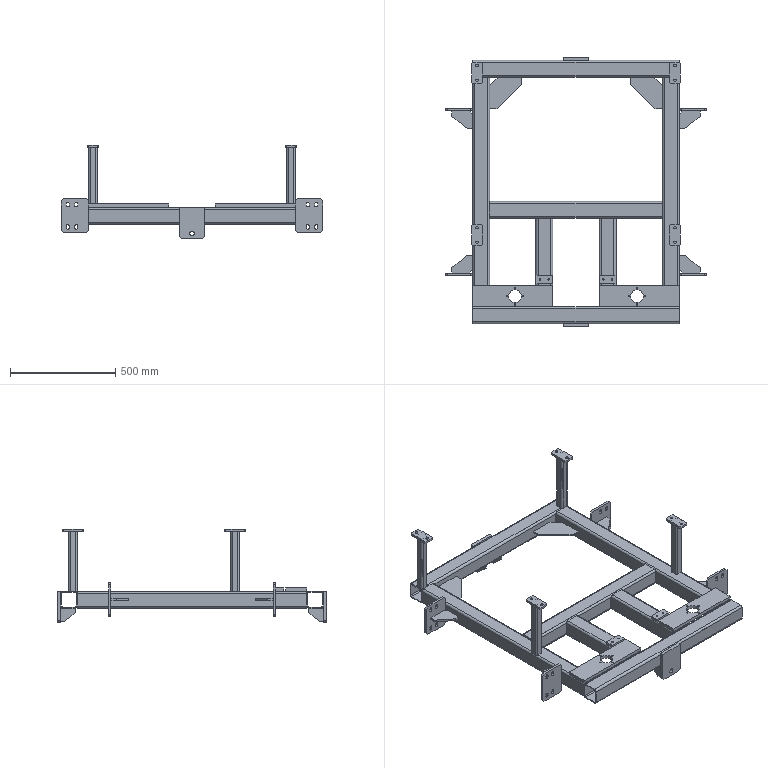Part | STEP file | 39 solids | 554 faces | box 1240 x 1282 x 445 mm | volume 12232636 mm3 | plane 362 | cylinder 184 | cone 8 | commonest cylinder face diameters 14 x48 10 x28 20 x28 6.8 x24 8 x16 12 x16